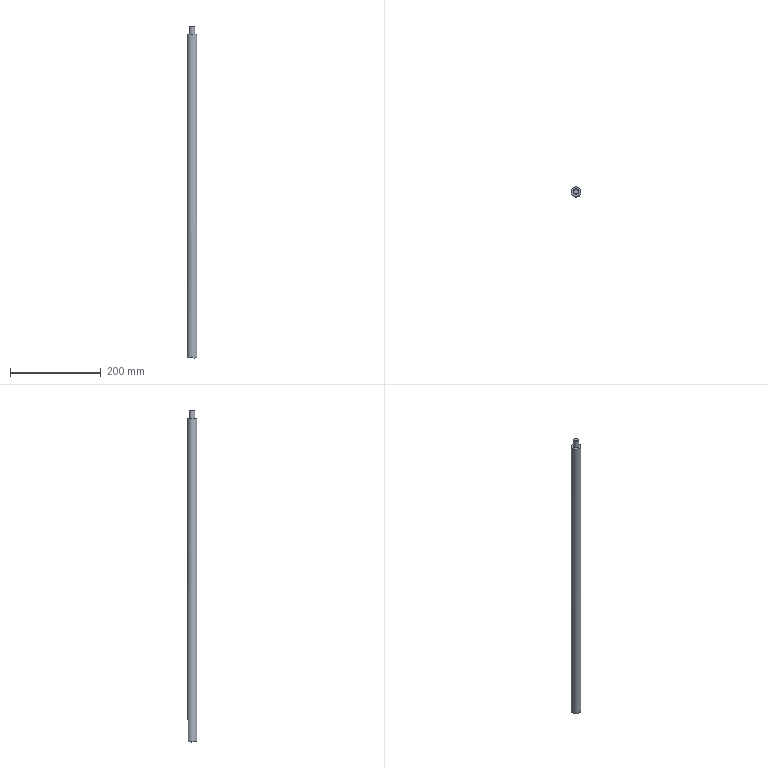Part | STEP file | solid 240 | 1 solid | 11 faces | box 22 x 22 x 730.955 mm | volume 269760 mm3 | plane 5 | cylinder 3 | cone 3 | commonest cylinder face diameters 10.2 x1 12 x1 22 x1